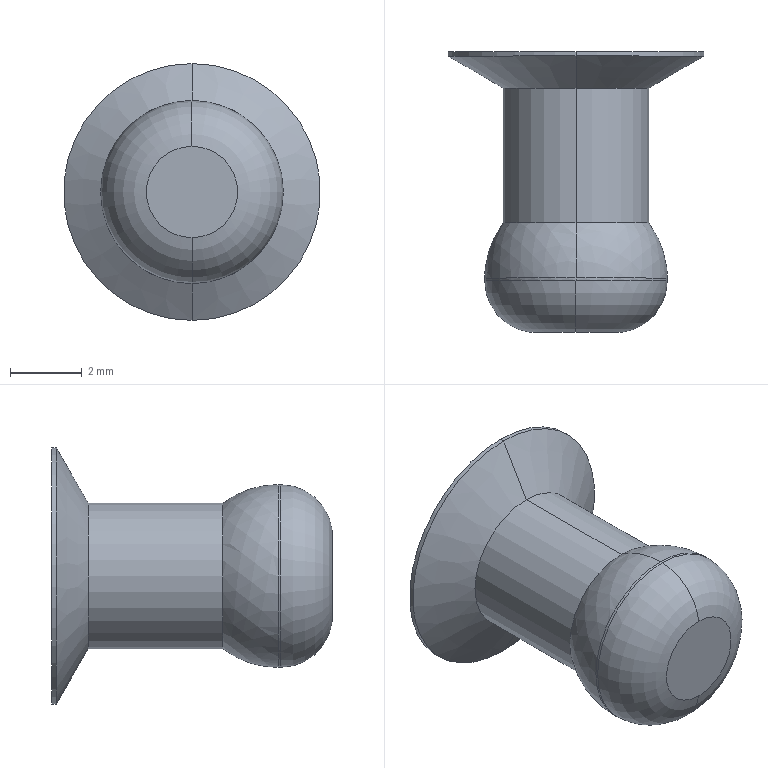Part | NX | features solid 2 | 1 solid | 17 faces | box 7.137 x 7.798 x 7.137 mm | volume 123.703 mm3 | cylinder 8 | plane 3 | torus 2 | sphere 2 | cone 2 | commonest cylinder face diameters 1.829 x2 4.039 x2 5.08 x2 7.137 x2
STEP:
#1=CARTESIAN_POINT('',(65.,2179.502,-994.13));
#2=VERTEX_POINT('',#1);
#3=CARTESIAN_POINT('',(65.,2179.502,-996.67));
#4=VERTEX_POINT('',#3);
#5=CARTESIAN_POINT('',(65.,2179.502,-995.4));
#6=DIRECTION('',(0.,1.,0.));
#7=DIRECTION('',(0.,0.,1.));
#8=AXIS2_PLACEMENT_3D('',#5,#6,#7);
#9=CIRCLE('',#8,1.27);
#10=EDGE_CURVE('',#2,#4,#9,.T.);
#11=ORIENTED_EDGE('',*,*,#10,.F.);
#12=CARTESIAN_POINT('',(65.,2179.502,-995.4));
#13=DIRECTION('',(0.,1.,0.));
#14=DIRECTION('',(0.,0.,-1.));
#15=AXIS2_PLACEMENT_3D('',#12,#13,#14);
#16=CIRCLE('',#15,1.27);
#17=EDGE_CURVE('',#4,#2,#16,.T.);
#18=ORIENTED_EDGE('',*,*,#17,.F.);
#19=EDGE_LOOP('',(#11,#18));
#20=FACE_BOUND('',#19,.T.);
#21=CARTESIAN_POINT('',(65.,2179.502,-995.4));
#22=DIRECTION('',(0.,-1.,0.));
#23=DIRECTION('',(0.,0.,-1.));
#24=AXIS2_PLACEMENT_3D('',#21,#22,#23);
#25=PLANE('',#24);
#26=ADVANCED_FACE('',(#20),#25,.T.);
#27=ORIENTED_EDGE('',*,*,#17,.T.);
#28=CARTESIAN_POINT('',(65.,2180.94,-992.86));
#29=VERTEX_POINT('',#28);
#30=CARTESIAN_POINT('',(65.,2180.94,-994.309));
#31=DIRECTION('',(1.,0.,0.000008994));
#32=DIRECTION('',(-0.000008994,0.,1.));
#33=AXIS2_PLACEMENT_3D('',#30,#31,#32);
#34=CIRCLE('',#33,1.449);
#35=EDGE_CURVE('',#2,#29,#34,.F.);
#36=ORIENTED_EDGE('',*,*,#35,.T.);
#37=CARTESIAN_POINT('',(65.,2180.94,-997.94));
#38=VERTEX_POINT('',#37);
#39=CARTESIAN_POINT('',(65.,2180.94,-995.4));
#40=DIRECTION('',(0.,1.,0.));
#41=DIRECTION('',(0.000002249,0.,-1.));
#42=AXIS2_PLACEMENT_3D('',#39,#40,#41);
#43=CIRCLE('',#42,2.54);
#44=EDGE_CURVE('',#38,#29,#43,.T.);
#45=ORIENTED_EDGE('',*,*,#44,.F.);
#46=CARTESIAN_POINT('',(65.,2180.94,-996.491));
#47=DIRECTION('',(-1.,0.,-0.000008996));
#48=DIRECTION('',(0.000008996,-0.000002409,-1.));
#49=AXIS2_PLACEMENT_3D('',#46,#47,#48);
#50=CIRCLE('',#49,1.449);
#51=EDGE_CURVE('',#38,#4,#50,.T.);
#52=ORIENTED_EDGE('',*,*,#51,.T.);
#53=EDGE_LOOP('',(#27,#36,#45,#52));
#54=FACE_BOUND('',#53,.T.);
#55=CARTESIAN_POINT('',(65.,2180.94,-995.4));
#56=DIRECTION('',(0.,-1.,0.));
#57=DIRECTION('',(1.,0.,0.));
#58=AXIS2_PLACEMENT_3D('',#55,#56,#57);
#59=DEGENERATE_TOROIDAL_SURFACE('',#58,1.091,1.449,.T.);
#60=ADVANCED_FACE('',(#54),#59,.T.);
#61=CARTESIAN_POINT('',(65.,2180.94,-995.4));
#62=DIRECTION('',(0.,1.,0.));
#63=DIRECTION('',(0.,0.,1.));
#64=AXIS2_PLACEMENT_3D('',#61,#62,#63);
#65=CIRCLE('',#64,2.54);
#66=EDGE_CURVE('',#29,#38,#65,.T.);
#67=ORIENTED_EDGE('',*,*,#66,.F.);
#68=ORIENTED_EDGE('',*,*,#35,.F.);
#69=ORIENTED_EDGE('',*,*,#10,.T.);
#70=ORIENTED_EDGE('',*,*,#51,.F.);
#71=EDGE_LOOP('',(#67,#68,#69,#70));
#72=FACE_BOUND('',#71,.T.);
#73=CARTESIAN_POINT('',(65.,2180.94,-995.4));
#74=DIRECTION('',(0.,-1.,0.));
#75=DIRECTION('',(0.,0.,1.));
#76=AXIS2_PLACEMENT_3D('',#73,#74,#75);
#77=DEGENERATE_TOROIDAL_SURFACE('',#76,1.091,1.449,.T.);
#78=ADVANCED_FACE('',(#72),#77,.T.);
#79=CARTESIAN_POINT('',(65.,2181.009,-997.94));
#80=VERTEX_POINT('',#79);
#81=CARTESIAN_POINT('',(65.,2181.009,-992.86));
#82=VERTEX_POINT('',#81);
#83=CARTESIAN_POINT('',(65.,2181.009,-995.4));
#84=DIRECTION('',(0.,-1.,0.));
#85=DIRECTION('',(0.000002249,0.,-1.));
#86=AXIS2_PLACEMENT_3D('',#83,#84,#85);
#87=CIRCLE('',#86,2.54);
#88=EDGE_CURVE('',#80,#82,#87,.T.);
#89=ORIENTED_EDGE('',*,*,#88,.T.);
#90=CARTESIAN_POINT('',(65.,2181.009,-992.86));
#91=DIRECTION('',(0.00008212,-1.,-0.000000002));
#92=VECTOR('',#91,1000.);
#93=LINE('',#90,#92);
#94=EDGE_CURVE('',#29,#82,#93,.F.);
#95=ORIENTED_EDGE('',*,*,#94,.F.);
#96=ORIENTED_EDGE('',*,*,#66,.T.);
#97=CARTESIAN_POINT('',(65.,2181.009,-997.94));
#98=DIRECTION('',(0.000000027,-1.,0.000000001));
#99=VECTOR('',#98,1000.);
#100=LINE('',#97,#99);
#101=EDGE_CURVE('',#80,#38,#100,.T.);
#102=ORIENTED_EDGE('',*,*,#101,.F.);
#103=EDGE_LOOP('',(#89,#95,#96,#102));
#104=FACE_BOUND('',#103,.T.);
#105=CARTESIAN_POINT('',(65.,2187.69,-995.4));
#106=DIRECTION('',(0.,-1.,0.));
#107=DIRECTION('',(0.,0.,-1.));
#108=AXIS2_PLACEMENT_3D('',#105,#106,#107);
#109=CYLINDRICAL_SURFACE('',#108,2.54);
#110=ADVANCED_FACE('',(#104),#109,.T.);
#111=ORIENTED_EDGE('',*,*,#44,.T.);
#112=ORIENTED_EDGE('',*,*,#94,.T.);
#113=CARTESIAN_POINT('',(65.,2181.009,-995.4));
#114=DIRECTION('',(0.,-1.,0.));
#115=DIRECTION('',(0.,0.,1.));
#116=AXIS2_PLACEMENT_3D('',#113,#114,#115);
#117=CIRCLE('',#116,2.54);
#118=EDGE_CURVE('',#82,#80,#117,.T.);
#119=ORIENTED_EDGE('',*,*,#118,.T.);
#120=ORIENTED_EDGE('',*,*,#101,.T.);
#121=EDGE_LOOP('',(#111,#112,#119,#120));
#122=FACE_BOUND('',#121,.T.);
#123=CARTESIAN_POINT('',(65.,2187.69,-995.4));
#124=DIRECTION('',(0.,-1.,0.));
#125=DIRECTION('',(0.,0.,-1.));
#126=AXIS2_PLACEMENT_3D('',#123,#124,#125);
#127=CYLINDRICAL_SURFACE('',#126,2.54);
#128=ADVANCED_FACE('',(#122),#127,.T.);
#129=ORIENTED_EDGE('',*,*,#118,.F.);
#130=CARTESIAN_POINT('',(65.,2182.55,-993.381));
#131=VERTEX_POINT('',#130);
#132=CARTESIAN_POINT('',(65.,2181.009,-995.4));
#133=DIRECTION('',(1.,0.,0.));
#134=DIRECTION('',(0.,0.6066,0.795));
#135=AXIS2_PLACEMENT_3D('',#132,#133,#134);
#136=CIRCLE('',#135,2.54);
#137=EDGE_CURVE('',#82,#131,#136,.F.);
#138=ORIENTED_EDGE('',*,*,#137,.T.);
#139=CARTESIAN_POINT('',(65.,2182.55,-997.419));
#140=VERTEX_POINT('',#139);
#141=CARTESIAN_POINT('',(65.,2182.55,-995.4));
#142=DIRECTION('',(0.,1.,0.));
#143=DIRECTION('',(0.,0.,-1.));
#144=AXIS2_PLACEMENT_3D('',#141,#142,#143);
#145=CIRCLE('',#144,2.019);
#146=EDGE_CURVE('',#140,#131,#145,.T.);
#147=ORIENTED_EDGE('',*,*,#146,.F.);
#148=CARTESIAN_POINT('',(65.,2181.009,-995.4));
#149=DIRECTION('',(-1.,0.,0.));
#150=DIRECTION('',(0.,0.6066,-0.795));
#151=AXIS2_PLACEMENT_3D('',#148,#149,#150);
#152=CIRCLE('',#151,2.54);
#153=EDGE_CURVE('',#140,#80,#152,.T.);
#154=ORIENTED_EDGE('',*,*,#153,.T.);
#155=EDGE_LOOP('',(#129,#138,#147,#154));
#156=FACE_BOUND('',#155,.T.);
#157=CARTESIAN_POINT('',(65.,2181.009,-995.4));
#158=DIRECTION('',(0.,0.6066,-0.795));
#159=DIRECTION('',(0.,0.795,0.6066));
#160=AXIS2_PLACEMENT_3D('',#157,#158,#159);
#161=SPHERICAL_SURFACE('',#160,2.54);
#162=ADVANCED_FACE('',(#156),#161,.T.);
#163=CARTESIAN_POINT('',(65.,2182.55,-995.4));
#164=DIRECTION('',(0.,1.,0.));
#165=DIRECTION('',(0.,0.,1.));
#166=AXIS2_PLACEMENT_3D('',#163,#164,#165);
#167=CIRCLE('',#166,2.019);
#168=EDGE_CURVE('',#131,#140,#167,.T.);
#169=ORIENTED_EDGE('',*,*,#168,.F.);
#170=ORIENTED_EDGE('',*,*,#137,.F.);
#171=ORIENTED_EDGE('',*,*,#88,.F.);
#172=ORIENTED_EDGE('',*,*,#153,.F.);
#173=EDGE_LOOP('',(#169,#170,#171,#172));
#174=FACE_BOUND('',#173,.T.);
#175=CARTESIAN_POINT('',(65.,2181.009,-995.4));
#176=DIRECTION('',(0.,0.6066,-0.795));
#177=DIRECTION('',(0.,0.795,0.6066));
#178=AXIS2_PLACEMENT_3D('',#175,#176,#177);
#179=SPHERICAL_SURFACE('',#178,2.54);
#180=ADVANCED_FACE('',(#174),#179,.T.);
#181=CARTESIAN_POINT('',(65.,2186.284,-997.419));
#182=VERTEX_POINT('',#181);
#183=CARTESIAN_POINT('',(65.,2186.284,-993.381));
#184=VERTEX_POINT('',#183);
#185=CARTESIAN_POINT('',(65.,2186.284,-995.4));
#186=DIRECTION('',(0.,-1.,0.));
#187=DIRECTION('',(0.,0.,-1.));
#188=AXIS2_PLACEMENT_3D('',#185,#186,#187);
#189=CIRCLE('',#188,2.019);
#190=EDGE_CURVE('',#182,#184,#189,.T.);
#191=ORIENTED_EDGE('',*,*,#190,.T.);
#192=CARTESIAN_POINT('',(65.,2186.284,-993.381));
#193=DIRECTION('',(0.,-1.,0.));
#194=VECTOR('',#193,1000.);
#195=LINE('',#192,#194);
#196=EDGE_CURVE('',#184,#131,#195,.T.);
#197=ORIENTED_EDGE('',*,*,#196,.T.);
#198=ORIENTED_EDGE('',*,*,#168,.T.);
#199=CARTESIAN_POINT('',(65.,2186.284,-997.419));
#200=DIRECTION('',(0.,-1.,0.));
#201=VECTOR('',#200,1000.);
#202=LINE('',#199,#201);
#203=EDGE_CURVE('',#140,#182,#202,.F.);
#204=ORIENTED_EDGE('',*,*,#203,.T.);
#205=EDGE_LOOP('',(#191,#197,#198,#204));
#206=FACE_BOUND('',#205,.T.);
#207=CARTESIAN_POINT('',(65.,2187.69,-995.4));
#208=DIRECTION('',(0.,-1.,0.));
#209=DIRECTION('',(0.,0.,-1.));
#210=AXIS2_PLACEMENT_3D('',#207,#208,#209);
#211=CYLINDRICAL_SURFACE('',#210,2.019);
#212=ADVANCED_FACE('',(#206),#211,.T.);
#213=ORIENTED_EDGE('',*,*,#146,.T.);
#214=ORIENTED_EDGE('',*,*,#196,.F.);
#215=CARTESIAN_POINT('',(65.,2186.284,-995.4));
#216=DIRECTION('',(0.,-1.,0.));
#217=DIRECTION('',(0.,0.,1.));
#218=AXIS2_PLACEMENT_3D('',#215,#216,#217);
#219=CIRCLE('',#218,2.019);
#220=EDGE_CURVE('',#184,#182,#219,.T.);
#221=ORIENTED_EDGE('',*,*,#220,.T.);
#222=ORIENTED_EDGE('',*,*,#203,.F.);
#223=EDGE_LOOP('',(#213,#214,#221,#222));
#224=FACE_BOUND('',#223,.T.);
#225=CARTESIAN_POINT('',(65.,2187.69,-995.4));
#226=DIRECTION('',(0.,-1.,0.));
#227=DIRECTION('',(0.,0.,-1.));
#228=AXIS2_PLACEMENT_3D('',#225,#226,#227);
#229=CYLINDRICAL_SURFACE('',#228,2.019);
#230=ADVANCED_FACE('',(#224),#229,.T.);
#231=ORIENTED_EDGE('',*,*,#220,.F.);
#232=CARTESIAN_POINT('',(65.,2187.179,-991.831));
#233=VERTEX_POINT('',#232);
#234=CARTESIAN_POINT('',(65.,2187.179,-991.831));
#235=DIRECTION('',(0.,-0.5,-0.866));
#236=VECTOR('',#235,1000.);
#237=LINE('',#234,#236);
#238=EDGE_CURVE('',#233,#184,#237,.T.);
#239=ORIENTED_EDGE('',*,*,#238,.F.);
#240=CARTESIAN_POINT('',(65.,2187.179,-998.969));
#241=VERTEX_POINT('',#240);
#242=CARTESIAN_POINT('',(65.,2187.179,-995.4));
#243=DIRECTION('',(0.,1.,0.));
#244=DIRECTION('',(0.,0.,-1.));
#245=AXIS2_PLACEMENT_3D('',#242,#243,#244);
#246=CIRCLE('',#245,3.569);
#247=EDGE_CURVE('',#241,#233,#246,.T.);
#248=ORIENTED_EDGE('',*,*,#247,.F.);
#249=CARTESIAN_POINT('',(65.,2187.179,-998.969));
#250=DIRECTION('',(0.,-0.5,0.866));
#251=VECTOR('',#250,1000.);
#252=LINE('',#249,#251);
#253=EDGE_CURVE('',#182,#241,#252,.F.);
#254=ORIENTED_EDGE('',*,*,#253,.F.);
#255=EDGE_LOOP('',(#231,#239,#248,#254));
#256=FACE_BOUND('',#255,.T.);
#257=CARTESIAN_POINT('',(65.,2186.731,-995.4));
#258=DIRECTION('',(0.,1.,0.));
#259=DIRECTION('',(0.,0.,1.));
#260=AXIS2_PLACEMENT_3D('',#257,#258,#259);
#261=CONICAL_SURFACE('',#260,2.794,1.047);
#262=ADVANCED_FACE('',(#256),#261,.T.);
#263=CARTESIAN_POINT('',(65.,2187.179,-995.4));
#264=DIRECTION('',(0.,1.,0.));
#265=DIRECTION('',(0.,0.,1.));
#266=AXIS2_PLACEMENT_3D('',#263,#264,#265);
#267=CIRCLE('',#266,3.569);
#268=EDGE_CURVE('',#233,#241,#267,.T.);
#269=ORIENTED_EDGE('',*,*,#268,.F.);
#270=ORIENTED_EDGE('',*,*,#238,.T.);
#271=ORIENTED_EDGE('',*,*,#190,.F.);
#272=ORIENTED_EDGE('',*,*,#253,.T.);
#273=EDGE_LOOP('',(#269,#270,#271,#272));
#274=FACE_BOUND('',#273,.T.);
#275=CARTESIAN_POINT('',(65.,2186.731,-995.4));
#276=DIRECTION('',(0.,1.,0.));
#277=DIRECTION('',(0.,0.,1.));
#278=AXIS2_PLACEMENT_3D('',#275,#276,#277);
#279=CONICAL_SURFACE('',#278,2.794,1.047);
#280=ADVANCED_FACE('',(#274),#279,.T.);
#281=CARTESIAN_POINT('',(65.,2187.3,-998.969));
#282=VERTEX_POINT('',#281);
#283=CARTESIAN_POINT('',(65.,2187.3,-991.831));
#284=VERTEX_POINT('',#283);
#285=CARTESIAN_POINT('',(65.,2187.3,-995.4));
#286=DIRECTION('',(0.,-1.,0.));
#287=DIRECTION('',(0.,0.,-1.));
#288=AXIS2_PLACEMENT_3D('',#285,#286,#287);
#289=CIRCLE('',#288,3.569);
#290=EDGE_CURVE('',#282,#284,#289,.T.);
#291=ORIENTED_EDGE('',*,*,#290,.T.);
#292=CARTESIAN_POINT('',(65.,2187.3,-991.831));
#293=DIRECTION('',(0.,-1.,0.));
#294=VECTOR('',#293,1000.);
#295=LINE('',#292,#294);
#296=EDGE_CURVE('',#284,#233,#295,.T.);
#297=ORIENTED_EDGE('',*,*,#296,.T.);
#298=ORIENTED_EDGE('',*,*,#268,.T.);
#299=CARTESIAN_POINT('',(65.,2187.3,-998.969));
#300=DIRECTION('',(0.,-1.,0.));
#301=VECTOR('',#300,1000.);
#302=LINE('',#299,#301);
#303=EDGE_CURVE('',#241,#282,#302,.F.);
#304=ORIENTED_EDGE('',*,*,#303,.T.);
#305=EDGE_LOOP('',(#291,#297,#298,#304));
#306=FACE_BOUND('',#305,.T.);
#307=CARTESIAN_POINT('',(65.,2187.69,-995.4));
#308=DIRECTION('',(0.,-1.,0.));
#309=DIRECTION('',(0.,0.,-1.));
#310=AXIS2_PLACEMENT_3D('',#307,#308,#309);
#311=CYLINDRICAL_SURFACE('',#310,3.569);
#312=ADVANCED_FACE('',(#306),#311,.T.);
#313=ORIENTED_EDGE('',*,*,#247,.T.);
#314=ORIENTED_EDGE('',*,*,#296,.F.);
#315=CARTESIAN_POINT('',(65.,2187.3,-995.4));
#316=DIRECTION('',(0.,-1.,0.));
#317=DIRECTION('',(0.,0.,1.));
#318=AXIS2_PLACEMENT_3D('',#315,#316,#317);
#319=CIRCLE('',#318,3.569);
#320=EDGE_CURVE('',#284,#282,#319,.T.);
#321=ORIENTED_EDGE('',*,*,#320,.T.);
#322=ORIENTED_EDGE('',*,*,#303,.F.);
#323=EDGE_LOOP('',(#313,#314,#321,#322));
#324=FACE_BOUND('',#323,.T.);
#325=CARTESIAN_POINT('',(65.,2187.69,-995.4));
#326=DIRECTION('',(0.,-1.,0.));
#327=DIRECTION('',(0.,0.,-1.));
#328=AXIS2_PLACEMENT_3D('',#325,#326,#327);
#329=CYLINDRICAL_SURFACE('',#328,3.569);
#330=ADVANCED_FACE('',(#324),#329,.T.);
#331=ORIENTED_EDGE('',*,*,#320,.F.);
#332=ORIENTED_EDGE('',*,*,#290,.F.);
#333=EDGE_LOOP('',(#331,#332));
#334=FACE_BOUND('',#333,.T.);
#335=CARTESIAN_POINT('',(65.,2187.3,-994.486));
#336=VERTEX_POINT('',#335);
#337=CARTESIAN_POINT('',(65.,2187.3,-996.314));
#338=VERTEX_POINT('',#337);
#339=CARTESIAN_POINT('',(65.,2187.3,-995.4));
#340=DIRECTION('',(0.,1.,0.));
#341=DIRECTION('',(0.,0.,1.));
#342=AXIS2_PLACEMENT_3D('',#339,#340,#341);
#343=CIRCLE('',#342,0.9144);
#344=EDGE_CURVE('',#336,#338,#343,.T.);
#345=ORIENTED_EDGE('',*,*,#344,.F.);
#346=CARTESIAN_POINT('',(65.,2187.3,-995.4));
#347=DIRECTION('',(0.,1.,0.));
#348=DIRECTION('',(0.,0.,-1.));
#349=AXIS2_PLACEMENT_3D('',#346,#347,#348);
#350=CIRCLE('',#349,0.9144);
#351=EDGE_CURVE('',#338,#336,#350,.T.);
#352=ORIENTED_EDGE('',*,*,#351,.F.);
#353=EDGE_LOOP('',(#345,#352));
#354=FACE_BOUND('',#353,.T.);
#355=CARTESIAN_POINT('',(65.,2187.3,-995.4));
#356=DIRECTION('',(0.,-1.,0.));
#357=DIRECTION('',(0.,0.,-1.));
#358=AXIS2_PLACEMENT_3D('',#355,#356,#357);
#359=PLANE('',#358);
#360=ADVANCED_FACE('',(#334,#354),#359,.F.);
#361=ORIENTED_EDGE('',*,*,#351,.T.);
#362=CARTESIAN_POINT('',(65.,2186.03,-994.486));
#363=VERTEX_POINT('',#362);
#364=CARTESIAN_POINT('',(65.,2186.03,-994.486));
#365=DIRECTION('',(0.,1.,0.));
#366=VECTOR('',#365,1000.);
#367=LINE('',#364,#366);
#368=EDGE_CURVE('',#363,#336,#367,.T.);
#369=ORIENTED_EDGE('',*,*,#368,.F.);
#370=CARTESIAN_POINT('',(65.,2186.03,-996.314));
#371=VERTEX_POINT('',#370);
#372=CARTESIAN_POINT('',(65.,2186.03,-995.4));
#373=DIRECTION('',(0.,-1.,0.));
#374=DIRECTION('',(0.,0.,1.));
#375=AXIS2_PLACEMENT_3D('',#372,#373,#374);
#376=CIRCLE('',#375,0.9144);
#377=EDGE_CURVE('',#363,#371,#376,.T.);
#378=ORIENTED_EDGE('',*,*,#377,.T.);
#379=CARTESIAN_POINT('',(65.,2186.03,-996.314));
#380=DIRECTION('',(0.,1.,0.));
#381=VECTOR('',#380,1000.);
#382=LINE('',#379,#381);
#383=EDGE_CURVE('',#338,#371,#382,.F.);
#384=ORIENTED_EDGE('',*,*,#383,.F.);
#385=EDGE_LOOP('',(#361,#369,#378,#384));
#386=FACE_BOUND('',#385,.T.);
#387=CARTESIAN_POINT('',(65.,2187.69,-995.4));
#388=DIRECTION('',(0.,-1.,0.));
#389=DIRECTION('',(0.,0.,-1.));
#390=AXIS2_PLACEMENT_3D('',#387,#388,#389);
#391=CYLINDRICAL_SURFACE('',#390,0.9144);
#392=ADVANCED_FACE('',(#386),#391,.F.);
#393=CARTESIAN_POINT('',(65.,2186.03,-995.4));
#394=DIRECTION('',(0.,-1.,0.));
#395=DIRECTION('',(0.,0.,-1.));
#396=AXIS2_PLACEMENT_3D('',#393,#394,#395);
#397=CIRCLE('',#396,0.9144);
#398=EDGE_CURVE('',#371,#363,#397,.T.);
#399=ORIENTED_EDGE('',*,*,#398,.T.);
#400=ORIENTED_EDGE('',*,*,#368,.T.);
#401=ORIENTED_EDGE('',*,*,#344,.T.);
#402=ORIENTED_EDGE('',*,*,#383,.T.);
#403=EDGE_LOOP('',(#399,#400,#401,#402));
#404=FACE_BOUND('',#403,.T.);
#405=CARTESIAN_POINT('',(65.,2187.69,-995.4));
#406=DIRECTION('',(0.,-1.,0.));
#407=DIRECTION('',(0.,0.,-1.));
#408=AXIS2_PLACEMENT_3D('',#405,#406,#407);
#409=CYLINDRICAL_SURFACE('',#408,0.9144);
#410=ADVANCED_FACE('',(#404),#409,.F.);
#411=ORIENTED_EDGE('',*,*,#398,.F.);
#412=ORIENTED_EDGE('',*,*,#377,.F.);
#413=EDGE_LOOP('',(#411,#412));
#414=FACE_BOUND('',#413,.T.);
#415=CARTESIAN_POINT('',(65.,2186.03,-995.4));
#416=DIRECTION('',(0.,-1.,0.));
#417=DIRECTION('',(0.,0.,-1.));
#418=AXIS2_PLACEMENT_3D('',#415,#416,#417);
#419=PLANE('',#418);
#420=ADVANCED_FACE('',(#414),#419,.F.);
#421=CLOSED_SHELL('',(#26,#60,#78,#110,#128,#162,#180,#212,#230,#262,#280,#312,#330,#360,#392,#410,#420));
#422=MANIFOLD_SOLID_BREP('',#421);
#423=(LENGTH_UNIT()NAMED_UNIT(*)SI_UNIT(.MILLI.,.METRE.));
#424=UNCERTAINTY_MEASURE_WITH_UNIT(LENGTH_MEASURE(0.00001),#423,'','');
#425=(NAMED_UNIT(*)PLANE_ANGLE_UNIT()SI_UNIT($,.RADIAN.));
#426=(NAMED_UNIT(*)SI_UNIT($,.STERADIAN.)SOLID_ANGLE_UNIT());
#427=(GEOMETRIC_REPRESENTATION_CONTEXT(3)GLOBAL_UNCERTAINTY_ASSIGNED_CONTEXT((#424))GLOBAL_UNIT_ASSIGNED_CONTEXT((#423,#425,#426))REPRESENTATION_CONTEXT('',''));
#428=ADVANCED_BREP_SHAPE_REPRESENTATION('',(#422),#427);